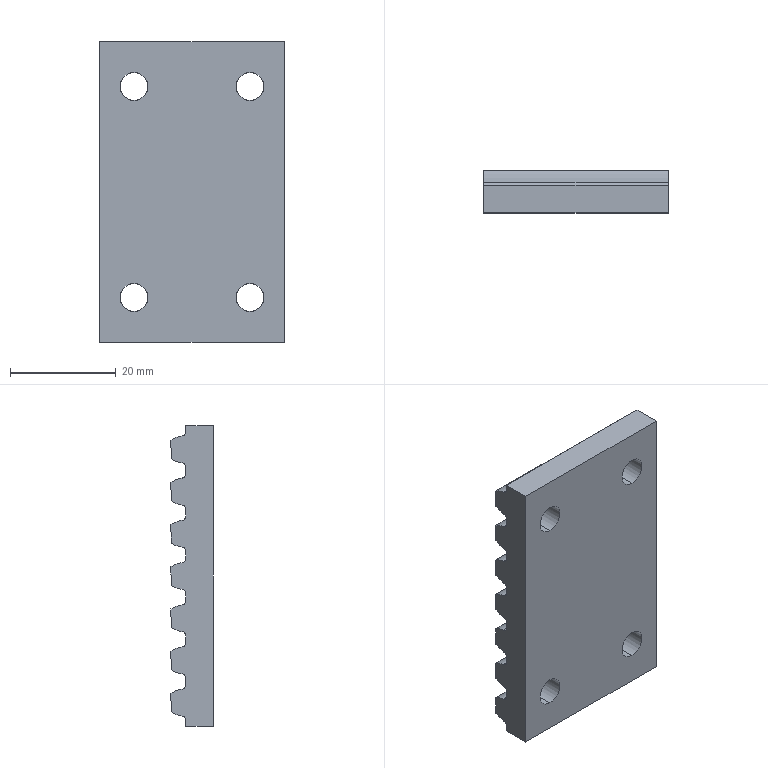Part | NX | features BREP 1 | 1 solid | 76 faces | box 35 x 8 x 57 mm | volume 13034 mm3 | cylinder 52 | plane 24 | commonest cylinder face diameters 1.6 x22 10.4 x22 5.3 x8